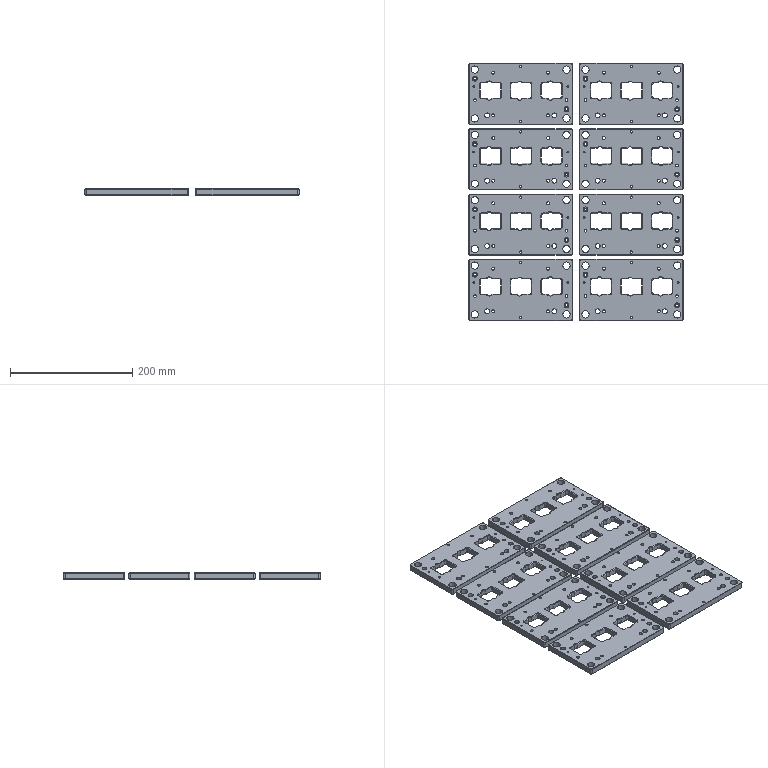NC program | NX | posted with a generic post | part box 351 x 421 x 10 mm
Whole program:
N10 G17 G21 G94 G90
(DRILLING_COPY , TOOL : D4A45)
N12 T02 M6
N14 G54
N16 G17 G0 G90 X0. Y45. S5000 M3
N18 G43 Z30. H2
N20 G94 G81 G98 Z-1. F250. R3.
N22 X45. Y35.
N24 X75. Y40.
N26 X77. Y12.
N28 X75. Y-10.
N30 Y-25.
N32 Y-40.
N34 X55. Y-35.
N36 X45.
N38 X0. Y-45.
N40 X-45. Y-35.
N42 X-55.
N44 X-75. Y-40.
N46 Y-10.
N48 X-77. Y12.
N50 X-75. Y25.
N52 Y40.
N54 X-45. Y35.
N56 G80
N58 G0 X-45. Y35. Z30.
N60 M5
(DRILLING_COPY_COPY_COPY_COPY , TOOL : 4.5ZT)
N62 T14 M6
N64 G54
N66 G17 G0 G90 X-75. Y25. S1910 M3
N68 G43 Z30. H14
N70 G94 G83 G98 Z-12.702 F180. Q2. R3.
N72 Y-10.
N74 X75.
N76 Y-25.
N78 G80
N80 G0 X75. Y-25. Z30.
(DRILLING_COPY_COPY_COPY_COPY_COPY , TOOL : 4.5ZT)
N82 X-45. Y-35.
N84 G83 Z-12.702 F180. Q2. R3.
N86 Y35.
N88 X45.
N90 Y-35.
N92 G80
N94 G0 X45. Y-35. Z30.
N96 M5
(DRILLING_COPY_COPY_COPY_COPY_COPY_COPY , TOOL : 2.5ZT)
N98 T12 M6
N100 G54
N102 G17 G0 G90 X77. Y12. S1910 M3
N104 G43 Z30. H12
N106 G94 G83 G98 Z-12.251 F180. Q2. R3.
N108 X-77.
N110 G80
N112 G0 X-77. Y12. Z30.
N114 M5
(ZLEVEL_PROFILE_1_COPY_1_COPY_COPY , TOOL : D4A45)
N116 T02 M6
N118 G54
N120 G17 G0 G90 X44.818 Y-35.693 S9500 M3
N122 G43 Z30. H2
N124 Z0.
N126 G94 G1 Z-1. F1000.
N128 X44.654 Y-36.316
N130 G3 X45. Y-36.516 R0.4
N132 G1 X45.004
N134 G3 X46.516 Y-34.996 R1.516
N136 X45. Y-36.516 R-1.516
N138 X45.346 Y-36.316 R0.4
N140 G1 X45.182 Y-35.693
N142 Z0.
N144 G0 Z30.
N146 X-45.182
N148 Z0.
N150 G1 Z-1.
N152 X-45.346 Y-36.316
N154 G3 X-45. Y-36.516 R0.4
N156 X-43.484 Y-35. R1.516
N158 X-45. Y-36.516 R-1.516
N160 X-44.654 Y-36.316 R0.4
N162 G1 X-44.818 Y-35.693
N164 Z0.
N166 G0 Z30.
N168 X45.182 Y35.693
N170 Z0.
N172 G1 Z-1.
N174 X45.346 Y36.316
N176 G3 X45. Y36.516 R0.4
N178 X43.484 Y35. R1.516
N180 X45. Y36.516 R-1.516
N182 X44.654 Y36.316 R0.4
N184 G1 X44.818 Y35.693
N186 Z0.
N188 G0 Z30.
N190 X-44.818
N192 Z0.
N194 G1 Z-1.
N196 X-44.654 Y36.316
N198 G3 X-45. Y36.516 R0.4
N200 G1 X-45.004
N202 G3 X-46.516 Y34.996 R1.516
N204 X-45. Y36.516 R-1.516
N206 X-45.346 Y36.316 R0.4
N208 G1 X-45.182 Y35.693
N210 Z0.
N212 G0 Z30.
N214 X54.228 Y-37.104
N216 Z0.
N218 G1 Z-1.
N220 X54.654 Y-37.841
N222 G3 X55. Y-38.041 R0.4
N224 G1 X55.006
N226 G3 X58.041 Y-34.994 R3.041
N228 X55. Y-38.041 R-3.041
N230 X55.346 Y-37.841 R0.4
N232 G1 X55.772 Y-37.104
N234 Z0.
N236 G0 Z30.
N238 X-55.772
N240 Z0.
N242 G1 Z-1.
N244 X-55.346 Y-37.841
N246 G3 X-55. Y-38.041 R0.4
N248 X-51.959 Y-35. R3.041
N250 X-55. Y-38.041 R-3.041
N252 X-54.654 Y-37.841 R0.4
N254 G1 X-54.228 Y-37.104
N256 Z0.
N258 G0 Z30.
N260 X77.291 Y12.
N262 Z1.
N264 G1 Z-1.
N266 G3 X77. Y12.291 R0.291
N268 X77.291 Y12. R-0.291
N270 X77.191 Y12.173 R0.2
N272 G1 Z0.
N274 G0 Z30.
N276 X-77.104 Y25.772
N278 Z0.
N280 G1 Z-1.
N282 X-77.841 Y25.346
N284 G3 X-78.041 Y25. R0.4
N286 X-75. Y21.959 R3.041
N288 X-78.041 Y25. R-3.041
N290 X-77.841 Y24.654 R0.4
N292 G1 X-77.104 Y24.228
N294 Z0.
N296 G0 Z30.
N298 X74.271 Y-44.178
N300 Z0.
N302 G1 Z-1.
N304 X74.654 Y-44.841
N306 G3 X75. Y-45.041 R0.4
N308 X80.041 Y-40. R5.041
N310 X75. Y-45.041 R-5.041
N312 X75.346 Y-44.841 R0.4
N314 G1 X75.729 Y-44.178
N316 Z0.
N318 G0 Z30.
N320 X16.412 Y-5.45
N322 Z0.
N324 G1 Z-1.
N326 X17.033 Y-5.596
N328 G3 X17.233 Y-5.25 R0.4
N330 G1 Y16.64
N332 G3 X15.689 Y18.213 R1.573
N334 G1 X15.639 Y18.221
N336 X2.794
N338 X2.442 Y18.215
N340 X2.395 Y18.183
N342 X1.596
N344 G2 X0.968 Y18.429 R0.994
N346 G3 X-4.447 Y18.426 R4.041
N348 G2 X-5.062 Y18.187 R0.927
N350 G1 X-5.787 Y18.183
N352 X-5.911 Y18.2
N354 X-5.917 Y18.21
N356 X-6.186 Y18.221
N358 X-14.716
N360 X-14.766 Y18.212
N362 G3 X-16.308 Y16.625 R1.57
N364 G1 Y-5.25
N366 G3 X-14.716 Y-6.843 R1.57
N368 G1 X-6.485 Y-6.844
N370 X-6.494 Y-6.825
N372 X-6.479 Y-6.81
N374 X-6.46 Y-6.818
N376 X-6.038 Y-6.825
N378 X-5.986 Y-6.84
N380 Y-6.818
N382 X-5.927 Y-6.799
N384 X-5.873 Y-6.837
N386 X-5.87 Y-6.9
N388 X-5.837 Y-6.927
N390 X-5.578 Y-7.25
N392 X-5.565 Y-7.3
N394 G3 X2.07 Y-7.321 R5.071
N396 G1 X2.088 Y-7.262
N398 X2.131 Y-7.216
N400 X2.245 Y-7.072
N402 X2.395 Y-6.896
N404 G2 X2.519 Y-6.837 R0.069
N406 G1 X2.569 Y-6.824
N408 X2.968 Y-6.816
N410 X2.987 Y-6.809
N412 X3.002 Y-6.825
N414 X2.993 Y-6.844
N416 X15.639 Y-6.843
N418 G3 X17.233 Y-5.25 R1.571
N420 X17.028 Y-4.907 R0.4
N422 G1 X16.433 Y-4.574
N424 Z0.
N426 G0 Z30.
N428 X-75.729 Y-44.178
N430 Z0.
N432 G1 Z-1.
N434 X-75.346 Y-44.841
N436 G3 X-75. Y-45.041 R0.4
N438 G1 X-74.998
N440 G3 X-69.959 Y-39.998 R5.041
N442 X-75. Y-45.041 R-5.041
N444 X-74.654 Y-44.841 R0.4
N446 G1 X-74.271 Y-44.178
N448 Z0.
N450 G0 Z30.
N452 X-0.092 Y-45.223
N454 Z0.
N456 G1 Z-1.
N458 X-0.346 Y-45.841
N460 G3 X0. Y-46.041 R0.4
N462 X1.041 Y-45. R1.041
N464 X0. Y-46.041 R-1.041
N466 X0.346 Y-45.841 R0.4
N468 G1 X0.092 Y-45.223
N470 Z0.
N472 G0 Z30.
N474 X-77.291 Y12.
N476 Z1.
N478 G1 Z-1.
N480 Y11.995
N482 G3 X-77.291 Y12. R-0.291
N484 X-77.191 Y11.827 R0.2
N486 G1 Z0.
N488 G0 Z30.
N490 X0.092 Y45.223
N492 Z0.
N494 G1 Z-1.
N496 X0.346 Y45.841
N498 G3 X0. Y46.041 R0.4
N500 X-1.041 Y45. R1.041
N502 X0. Y46.041 R-1.041
N504 X-0.346 Y45.841 R0.4
N506 G1 X-0.092 Y45.223
N508 Z0.
N510 G0 Z30.
N512 X34.515 Y15.004
N514 Z0.
N516 G1 Z-1.
N518 X34.013 Y14.91
N520 G3 X33.709 Y14.65 R0.4
N522 G1 X33.692 Y14.6
N524 Y-3.325
N526 G3 X37.265 Y-6.843 R3.57
N528 G1 X43.501
N530 X43.526 Y-6.848
N532 X43.518 Y-6.83
N534 X43.531 Y-6.814
N536 X43.551 Y-6.817
N538 X43.777 Y-6.825
N540 G2 X44. Y-6.835 R0.388
N542 G1 X44.041 Y-6.806
N544 X44.092 Y-6.813
N546 X44.124 Y-6.851
N548 X44.128 Y-6.895
N550 X44.174 Y-6.937
N552 X44.387 Y-7.2
N554 X44.431 Y-7.251
N556 X44.449 Y-7.315
N558 G3 X52.081 Y-7.308 R5.071
N560 G2 X52.251 Y-7.073 R0.585
N562 X52.394 Y-6.9 R0.451
N564 G1 X52.397 Y-6.84
N566 X52.446 Y-6.8
N568 X52.505 Y-6.811
N570 Y-6.825
N572 G3 X52.954 Y-6.816 R205.052
N574 G1 X53.004 Y-6.836
N576 Y-6.848
N578 X53.029 Y-6.843
N580 X63.663
N582 G3 X67.232 Y-3.291 R3.569
N584 G1 X67.207 Y-3.279
N586 X67.215 Y-3.248
N588 X67.243 Y-3.25
N590 Y14.625
N592 X67.234 Y14.65
N594 G3 X63.68 Y18.213 R3.573
N596 G1 X63.655 Y18.221
N598 X53.478
N600 X53.079 Y18.212
N602 Y18.2
N604 G2 X52.561 Y18.2 R2.252
N606 G1 X52.555 Y18.192
N608 X52.501 Y18.176
N610 X52.453 Y18.213
N612 X52.456 Y18.27
N614 G2 X52.308 Y18.452 R0.454
N616 G1 X52.285 Y18.475
N618 X52.167 Y18.625
N620 X52.156 Y18.642
N622 X52.163 Y18.677
N624 X52.136 Y18.7
N626 G3 X44.374 Y18.683 R5.072
N628 G2 X44.215 Y18.451 R0.507
N630 X44.075 Y18.274 R0.452
N632 G1 X44.066 Y18.25
N634 X44.07 Y18.225
N636 X44.043 Y18.18
N638 X43.989 Y18.172
N640 X43.95 Y18.207
N642 X43.927 Y18.2
N644 X43.75 Y18.186
N646 X43.715 Y18.197
N648 X43.501 Y18.184
N650 X43.465 Y18.2
N652 X43.102 Y18.221
N654 X37.265
N656 X37.24 Y18.212
N658 X37.165 Y18.211
N660 G3 X33.691 Y14.675 R3.571
N662 G1 X33.709 Y14.65
N664 G3 X34.074 Y14.485 R0.4
N666 G1 X34.515 Y14.528
N668 Z0.
N670 G0 Z30.
N672 X-65.485 Y16.838
N674 Z0.
N676 G1 Z-1.
N678 X-66.108 Y16.997
N680 G3 X-66.308 Y16.651 R0.4
N682 G1 Y-5.25
N684 G3 X-64.728 Y-6.843 R1.569
N686 G1 X-56.471 Y-6.844
N688 Y-6.831
N690 X-56.421 Y-6.815
N692 G3 X-56.097 Y-6.815 R2.9
N694 G1 X-55.997 Y-6.836
N696 X-55.942 Y-6.797
N698 X-55.877 Y-6.828
N700 X-55.873 Y-6.895
N702 X-55.823 Y-6.939
N704 X-55.578 Y-7.25
N706 X-55.573 Y-7.291
N708 G3 X-47.916 Y-7.305 R5.072
N710 G2 X-47.791 Y-7.114 R0.46
N712 G1 X-47.753 Y-7.075
N714 X-47.638 Y-6.925
N716 X-47.606 Y-6.9
N718 X-47.602 Y-6.839
N720 X-47.552 Y-6.8
N722 X-47.492 Y-6.811
N724 X-47.49 Y-6.825
N726 X-47.417 Y-6.821
N728 X-47.018 Y-6.817
N730 X-46.999 Y-6.81
N732 X-46.985 Y-6.825
N734 X-46.993 Y-6.844
N736 X-34.347 Y-6.843
N738 G3 X-32.767 Y-5.25 R1.571
N740 G1 Y16.
N742 X-32.755 Y16.4
N744 G3 X-32.774 Y16.8 R3.199
N746 X-34.322 Y18.213 R1.573
N748 G1 X-34.347 Y18.221
N750 X-46.694
N752 G2 X-47.442 Y18.197 R3.772
N754 G1 X-47.467 Y18.179
N756 X-47.523 Y18.175
N758 X-47.563 Y18.22
N760 X-47.552 Y18.275
N762 X-47.582 Y18.3
N764 X-47.841 Y18.637
N766 X-47.836 Y18.674
N768 X-47.864 Y18.7
N770 G3 X-55.623 Y18.686 R5.071
N772 G1 X-55.631 Y18.65
N774 X-55.773 Y18.463
N776 G2 X-55.934 Y18.25 R1.249
N778 G1 X-55.936 Y18.193
N780 X-55.99 Y18.167
N782 X-56.036 Y18.2
N784 G2 X-56.671 Y18.213 R2.696
N786 G1 X-57.07 Y18.221
N788 X-64.728
N790 X-64.753 Y18.213
N792 X-64.85 Y18.207
N794 G3 X-66.308 Y16.651 R1.559
N796 X-66.108 Y16.304 R0.4
N798 G1 X-65.508 Y15.958
N800 Z0.
N802 G0 Z30.
N804 X75.729 Y44.178
N806 Z0.
N808 G1 Z-1.
N810 X75.346 Y44.841
N812 G3 X75. Y45.041 R0.4
N814 G1 X74.998
N816 G3 X69.959 Y39.998 R5.041
N818 X75. Y45.041 R-5.041
N820 X74.654 Y44.841 R0.4
N822 G1 X74.271 Y44.178
N824 Z0.
N826 G0 Z30.
N828 X75.468 Y-10.149
N830 Z0.
N832 G1 Z-1.
N834 X76.091 Y-10.346
N836 G3 X76.291 Y-10. R0.4
N838 X75. Y-8.709 R1.291
N840 X76.291 Y-10. R-1.291
N842 X76.091 Y-9.654 R0.4
N844 G1 X75.468 Y-9.851
N846 Z0.
N848 G0 Z30.
N850 X-75.468
N852 Z0.
N854 G1 Z-1.
N856 X-76.091 Y-9.654
N858 G3 X-76.291 Y-10. R0.4
N860 X-75. Y-11.291 R1.291
N862 X-76.291 Y-10. R-1.291
N864 X-76.091 Y-10.346 R0.4
N866 G1 X-75.468 Y-10.149
N868 Z0.
N870 G0 Z30.
N872 X-79.178 Y40.729
N874 Z0.
N876 G1 Z-1.
N878 X-79.841 Y40.346
N880 G3 X-80.041 Y40. R0.4
N882 X-75. Y34.959 R5.041
N884 X-80.041 Y40. R-5.041
N886 X-79.841 Y39.654 R0.4
N888 G1 X-79.178 Y39.271
N890 Z0.
N892 G0 Z30.
N894 X77.104 Y-25.772
N896 Z0.
N898 G1 Z-1.
N900 X77.841 Y-25.346
N902 G3 X78.041 Y-25. R0.4
N904 X75. Y-21.959 R3.041
N906 X78.041 Y-25. R-3.041
N908 X77.841 Y-24.654 R0.4
N910 G1 X77.104 Y-24.228
N912 Z0.
N914 G0 Z30.
N916 X83.159 Y-51.2
N918 Z0.
N920 G1 Z-1.
N922 X82.846 Y-50.659
N924 G3 X82.5 Y-50.459 R0.4
N926 G1 X-82.5
N928 G2 X-85.459 Y-47.5 R2.959
N930 G1 Y47.5
N932 G2 X-82.5 Y50.459 R2.959
N934 G1 X82.5
N936 G2 X85.459 Y47.5 R2.959
N938 G1 Y-47.5
N940 G2 X82.5 Y-50.459 R2.959
N942 G3 X82.154 Y-50.659 R0.4
N944 G1 X81.807 Y-51.259
N946 Z0.
N948 G0 Z30.
N950 M5
(刀补 , TOOL : D3)
N952 T03 M6
N954 G54
N956 G17 G0 G90 X-45. Y35. S9500 M3
N958 G43 Z30. H3
N960 Z0.5
N962 G41 G94 G1 X-44.996 Y34.9 F1000. D3
N964 G3 X-44.075 Y35. R0.466
N966 X-44.075 Y35. Z-1. I-0.925 J0.
N968 X-44.075 Y35. Z-2.5 I-0.925 J0.
N970 X-44.075 Y35. Z-4. I-0.925 J0.
N972 X-44.075 Y35. Z-5.5 I-0.925 J0.
N974 X-44.075 Y35. Z-7. I-0.925 J0.
N976 X-44.075 Y35. Z-8.5 I-0.925 J0.
N978 X-44.075 Y35. Z-10. I-0.925 J0.
N980 X-45. Y35.925 R0.925
N982 X-44.075 Y35. R-0.925
N984 X-44.996 Y35.1 R0.466
N986 G40
N988 G1 X-45. Y35.
N990 G0 Z30.
N992 Y-35.
N994 Z0.5
N996 G41 G1 X-44.996 Y-35.1
N998 G3 X-44.075 Y-35. R0.466
N1000 X-44.075 Y-35. Z-1. I-0.925 J0.
N1002 X-44.075 Y-35. Z-2.5 I-0.925 J0.
N1004 X-44.075 Y-35. Z-4. I-0.925 J0.
N1006 X-44.075 Y-35. Z-5.5 I-0.925 J0.
N1008 X-44.075 Y-35. Z-7. I-0.925 J0.
N1010 X-44.075 Y-35. Z-8.5 I-0.925 J0.
N1012 X-44.075 Y-35. Z-10. I-0.925 J0.
N1014 X-45. Y-34.075 R0.925
N1016 X-44.075 Y-35. R-0.925
N1018 X-44.996 Y-34.9 R0.466
N1020 G40
N1022 G1 X-45. Y-35.
N1024 G0 Z30.
N1026 X45. Y35.
N1028 Z0.5
N1030 G41 G1 X45.004 Y34.9
N1032 G3 X45.925 Y35. R0.466
N1034 X45.925 Y35. Z-1. I-0.925 J0.
N1036 X45.925 Y35. Z-2.5 I-0.925 J0.
N1038 X45.925 Y35. Z-4. I-0.925 J0.
N1040 X45.925 Y35. Z-5.5 I-0.925 J0.
N1042 X45.925 Y35. Z-7. I-0.925 J0.
N1044 X45.925 Y35. Z-8.5 I-0.925 J0.
N1046 X45.925 Y35. Z-10. I-0.925 J0.
N1048 X45. Y35.925 R0.925
N1050 X45.925 Y35. R-0.925
N1052 X45.004 Y35.1 R0.466
N1054 G40
N1056 G1 X45. Y35.
N1058 G0 Z30.
N1060 Y-35.
N1062 Z0.5
N1064 G41 G1 X45.004 Y-35.1
N1066 G3 X45.925 Y-35. R0.466
N1068 X45.925 Y-35. Z-1. I-0.925 J0.
N1070 X45.925 Y-35. Z-2.5 I-0.925 J0.
N1072 X45.925 Y-35. Z-4. I-0.925 J0.
N1074 X45.925 Y-35. Z-5.5 I-0.925 J0.
N1076 X45.925 Y-35. Z-7. I-0.925 J0.
N1078 X45.925 Y-35. Z-8.5 I-0.925 J0.
N1080 X45.925 Y-35. Z-10. I-0.925 J0.
N1082 X45. Y-34.075 R0.925
N1084 X45.925 Y-35. R-0.925
N1086 X45.004 Y-34.9 R0.466
N1088 G40
N1090 G1 X45. Y-35.
N1092 G0 Z30.
N1094 X0. Y45.
N1096 Z0.5
N1098 G41 G1 X0.027 Y44.904
N1100 G3 X0.45 Y45. R0.222
N1102 X0.45 Y45. Z-1. I-0.45 J0.
N1104 X0.45 Y45. Z-2.5 I-0.45 J0.
N1106 X0.45 Y45. Z-4. I-0.45 J0.
N1108 X0.45 Y45. Z-5.5 I-0.45 J0.
N1110 X0.45 Y45. Z-7. I-0.45 J0.
N1112 X0.45 Y45. Z-8.5 I-0.45 J0.
N1114 X0.45 Y45. Z-10. I-0.45 J0.
N1116 X0. Y45.45 R0.45
N1118 X0.45 Y45. R-0.45
N1120 X0.027 Y45.096 R0.222
N1122 G40
N1124 G1 X0. Y45.
N1126 G0 Z30.
N1128 Y-45.
N1130 Z0.5
N1132 G41 G1 X0.027 Y-45.096
N1134 G3 X0.45 Y-45. R0.222
N1136 X0.45 Y-45. Z-1. I-0.45 J0.
N1138 X0.45 Y-45. Z-2.5 I-0.45 J0.
N1140 X0.45 Y-45. Z-4. I-0.45 J0.
N1142 X0.45 Y-45. Z-5.5 I-0.45 J0.
N1144 X0.45 Y-45. Z-7. I-0.45 J0.
N1146 X0.45 Y-45. Z-8.5 I-0.45 J0.
N1148 X0.45 Y-45. Z-10. I-0.45 J0.
N1150 X0. Y-44.55 R0.45
N1152 X0.45 Y-45. R-0.45
N1154 X0.027 Y-44.904 R0.222
N1156 G40
N1158 G1 X0. Y-45.
N1160 G0 Z30.
N1162 M5
N1164 M2